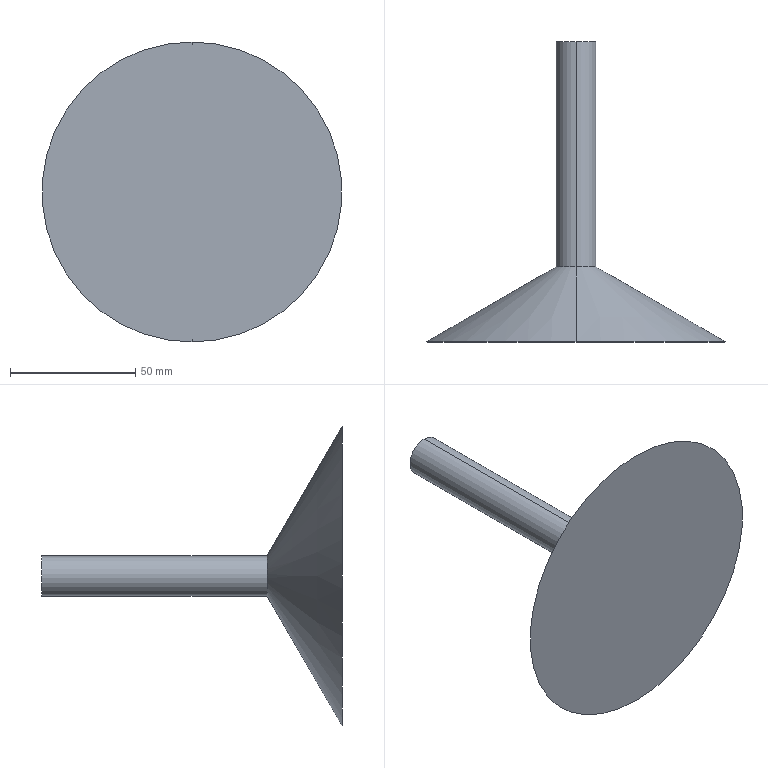Part | 1 solid | 6 faces | box 119.923 x 120 x 119.923 mm | volume 148128 mm3 | cylinder 2 | cone 2 | plane 2 | commonest cylinder face diameters 16 x2
STEP:
#1=CARTESIAN_POINT('',(0.,-1.44,8.));
#2=VERTEX_POINT('',#1);
#3=CARTESIAN_POINT('',(0.,-1.44,-8.));
#4=VERTEX_POINT('',#3);
#5=CARTESIAN_POINT('',(0.,-1.44,0.));
#6=DIRECTION('',(0.,1.,0.));
#7=DIRECTION('',(0.,0.,1.));
#8=AXIS2_PLACEMENT_3D('',#5,#6,#7);
#9=CIRCLE('',#8,8.);
#10=EDGE_CURVE('',#2,#4,#9,.T.);
#11=ORIENTED_EDGE('',*,*,#10,.T.);
#12=CARTESIAN_POINT('',(0.,88.56,-8.));
#13=VERTEX_POINT('',#12);
#14=CARTESIAN_POINT('',(0.,88.56,-8.));
#15=DIRECTION('',(0.,1.,0.));
#16=VECTOR('',#15,1000.);
#17=LINE('',#14,#16);
#18=EDGE_CURVE('',#4,#13,#17,.T.);
#19=ORIENTED_EDGE('',*,*,#18,.T.);
#20=CARTESIAN_POINT('',(0.,88.56,8.));
#21=VERTEX_POINT('',#20);
#22=CARTESIAN_POINT('',(0.,88.56,0.));
#23=DIRECTION('',(0.,1.,0.));
#24=DIRECTION('',(0.,0.,1.));
#25=AXIS2_PLACEMENT_3D('',#22,#23,#24);
#26=CIRCLE('',#25,8.);
#27=EDGE_CURVE('',#21,#13,#26,.T.);
#28=ORIENTED_EDGE('',*,*,#27,.F.);
#29=CARTESIAN_POINT('',(0.,88.56,8.));
#30=DIRECTION('',(0.,1.,0.));
#31=VECTOR('',#30,1000.);
#32=LINE('',#29,#31);
#33=EDGE_CURVE('',#2,#21,#32,.T.);
#34=ORIENTED_EDGE('',*,*,#33,.F.);
#35=EDGE_LOOP('',(#11,#19,#28,#34));
#36=FACE_OUTER_BOUND('',#35,.T.);
#37=CARTESIAN_POINT('',(0.,88.56,0.));
#38=DIRECTION('',(0.,1.,0.));
#39=DIRECTION('',(0.,0.,1.));
#40=AXIS2_PLACEMENT_3D('',#37,#38,#39);
#41=CYLINDRICAL_SURFACE('',#40,8.);
#42=ADVANCED_FACE('',(#36),#41,.T.);
#43=ORIENTED_EDGE('',*,*,#10,.F.);
#44=CARTESIAN_POINT('',(0.,-31.44,59.962));
#45=VERTEX_POINT('',#44);
#46=CARTESIAN_POINT('',(0.,-1.44,8.));
#47=DIRECTION('',(0.,-0.5,0.866));
#48=VECTOR('',#47,1000.);
#49=LINE('',#46,#48);
#50=EDGE_CURVE('',#2,#45,#49,.T.);
#51=ORIENTED_EDGE('',*,*,#50,.T.);
#52=CARTESIAN_POINT('',(0.,-31.44,-59.962));
#53=VERTEX_POINT('',#52);
#54=CARTESIAN_POINT('',(0.,-31.44,0.));
#55=DIRECTION('',(0.,1.,0.));
#56=DIRECTION('',(0.,0.,1.));
#57=AXIS2_PLACEMENT_3D('',#54,#55,#56);
#58=CIRCLE('',#57,59.962);
#59=EDGE_CURVE('',#45,#53,#58,.T.);
#60=ORIENTED_EDGE('',*,*,#59,.T.);
#61=CARTESIAN_POINT('',(0.,-1.44,-8.));
#62=DIRECTION('',(0.,-0.5,-0.866));
#63=VECTOR('',#62,1000.);
#64=LINE('',#61,#63);
#65=EDGE_CURVE('',#4,#53,#64,.T.);
#66=ORIENTED_EDGE('',*,*,#65,.F.);
#67=EDGE_LOOP('',(#43,#51,#60,#66));
#68=FACE_OUTER_BOUND('',#67,.T.);
#69=CARTESIAN_POINT('',(0.,-1.44,0.));
#70=DIRECTION('',(0.,-1.,0.));
#71=DIRECTION('',(0.,0.,-1.));
#72=AXIS2_PLACEMENT_3D('',#69,#70,#71);
#73=CONICAL_SURFACE('',#72,8.,1.047);
#74=ADVANCED_FACE('',(#68),#73,.T.);
#75=ORIENTED_EDGE('',*,*,#27,.T.);
#76=CARTESIAN_POINT('',(0.,88.56,0.));
#77=DIRECTION('',(0.,1.,0.));
#78=DIRECTION('',(0.,0.,1.));
#79=AXIS2_PLACEMENT_3D('',#76,#77,#78);
#80=CIRCLE('',#79,8.);
#81=EDGE_CURVE('',#13,#21,#80,.T.);
#82=ORIENTED_EDGE('',*,*,#81,.T.);
#83=EDGE_LOOP('',(#75,#82));
#84=FACE_OUTER_BOUND('',#83,.T.);
#85=CARTESIAN_POINT('',(-8.,88.56,0.));
#86=DIRECTION('',(0.,1.,0.));
#87=DIRECTION('',(0.,0.,1.));
#88=AXIS2_PLACEMENT_3D('',#85,#86,#87);
#89=PLANE('',#88);
#90=ADVANCED_FACE('',(#84),#89,.T.);
#91=CARTESIAN_POINT('',(0.,-31.44,0.));
#92=DIRECTION('',(0.,1.,0.));
#93=DIRECTION('',(0.,0.,1.));
#94=AXIS2_PLACEMENT_3D('',#91,#92,#93);
#95=CIRCLE('',#94,59.962);
#96=EDGE_CURVE('',#53,#45,#95,.T.);
#97=ORIENTED_EDGE('',*,*,#96,.F.);
#98=ORIENTED_EDGE('',*,*,#59,.F.);
#99=EDGE_LOOP('',(#97,#98));
#100=FACE_OUTER_BOUND('',#99,.T.);
#101=CARTESIAN_POINT('',(0.,-31.44,0.));
#102=DIRECTION('',(0.,-1.,0.));
#103=DIRECTION('',(0.,0.,-1.));
#104=AXIS2_PLACEMENT_3D('',#101,#102,#103);
#105=PLANE('',#104);
#106=ADVANCED_FACE('',(#100),#105,.T.);
#107=ORIENTED_EDGE('',*,*,#50,.F.);
#108=CARTESIAN_POINT('',(0.,-1.44,0.));
#109=DIRECTION('',(0.,1.,0.));
#110=DIRECTION('',(0.,0.,1.));
#111=AXIS2_PLACEMENT_3D('',#108,#109,#110);
#112=CIRCLE('',#111,8.);
#113=EDGE_CURVE('',#4,#2,#112,.T.);
#114=ORIENTED_EDGE('',*,*,#113,.F.);
#115=ORIENTED_EDGE('',*,*,#65,.T.);
#116=ORIENTED_EDGE('',*,*,#96,.T.);
#117=EDGE_LOOP('',(#107,#114,#115,#116));
#118=FACE_OUTER_BOUND('',#117,.T.);
#119=CARTESIAN_POINT('',(0.,-1.44,0.));
#120=DIRECTION('',(0.,-1.,0.));
#121=DIRECTION('',(0.,0.,-1.));
#122=AXIS2_PLACEMENT_3D('',#119,#120,#121);
#123=CONICAL_SURFACE('',#122,8.,1.047);
#124=ADVANCED_FACE('',(#118),#123,.T.);
#125=ORIENTED_EDGE('',*,*,#18,.F.);
#126=ORIENTED_EDGE('',*,*,#113,.T.);
#127=ORIENTED_EDGE('',*,*,#33,.T.);
#128=ORIENTED_EDGE('',*,*,#81,.F.);
#129=EDGE_LOOP('',(#125,#126,#127,#128));
#130=FACE_OUTER_BOUND('',#129,.T.);
#131=CARTESIAN_POINT('',(0.,88.56,0.));
#132=DIRECTION('',(0.,1.,0.));
#133=DIRECTION('',(0.,0.,1.));
#134=AXIS2_PLACEMENT_3D('',#131,#132,#133);
#135=CYLINDRICAL_SURFACE('',#134,8.);
#136=ADVANCED_FACE('',(#130),#135,.T.);
#137=CLOSED_SHELL('',(#42,#74,#90,#106,#124,#136));
#138=MANIFOLD_SOLID_BREP('',#137);
#139=CARTESIAN_POINT('',(0.,0.,0.));
#140=DIRECTION('',(0.,0.,1.));
#141=DIRECTION('',(1.,0.,0.));
#142=AXIS2_PLACEMENT_3D('',#139,#140,#141);
#143=(LENGTH_UNIT()NAMED_UNIT(*)SI_UNIT(.MILLI.,.METRE.));
#144=UNCERTAINTY_MEASURE_WITH_UNIT(LENGTH_MEASURE(0.00001),#143,'','');
#145=(NAMED_UNIT(*)PLANE_ANGLE_UNIT()SI_UNIT($,.RADIAN.));
#146=(NAMED_UNIT(*)SI_UNIT($,.STERADIAN.)SOLID_ANGLE_UNIT());
#147=(GEOMETRIC_REPRESENTATION_CONTEXT(3)GLOBAL_UNCERTAINTY_ASSIGNED_CONTEXT((#144))GLOBAL_UNIT_ASSIGNED_CONTEXT((#143,#145,#146))REPRESENTATION_CONTEXT('',''));
#148=ADVANCED_BREP_SHAPE_REPRESENTATION('',(#138,#142),#147);